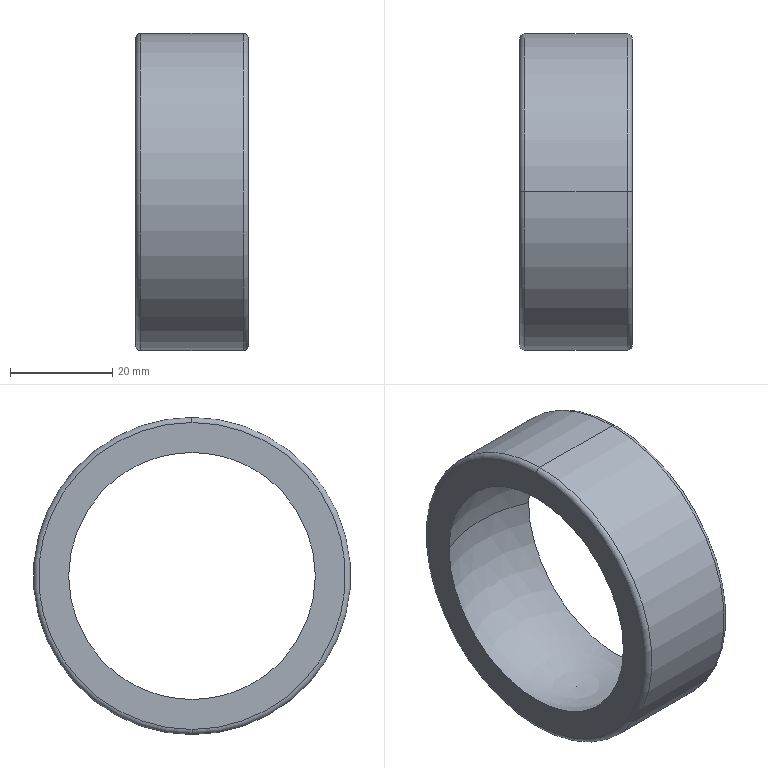Part | SolidWorks | features Fillet 1, Revolution 1 | 1 solid | 10 faces | box 22 x 62 x 62 mm | volume 20588 mm3 | torus 4 | sphere 2 | cylinder 2 | plane 2 | commonest cylinder face diameters 62 x2
STEP:
#1=CARTESIAN_POINT('',(11.,0.,-30.));
#2=VERTEX_POINT('',#1);
#3=CARTESIAN_POINT('',(11.,0.,30.));
#4=VERTEX_POINT('',#3);
#5=CARTESIAN_POINT('',(11.,0.,0.));
#6=DIRECTION('',(1.,0.,0.));
#7=DIRECTION('',(0.,0.,1.));
#8=AXIS2_PLACEMENT_3D('',#5,#6,#7);
#9=CIRCLE('',#8,30.);
#10=EDGE_CURVE('',#2,#4,#9,.T.);
#11=ORIENTED_EDGE('',*,*,#10,.F.);
#12=CARTESIAN_POINT('',(10.,0.,-31.));
#13=VERTEX_POINT('',#12);
#14=CARTESIAN_POINT('',(10.,0.,-30.));
#15=DIRECTION('',(0.,1.,0.));
#16=DIRECTION('',(0.,0.,1.));
#17=AXIS2_PLACEMENT_3D('',#14,#15,#16);
#18=CIRCLE('',#17,1.);
#19=EDGE_CURVE('',#2,#13,#18,.T.);
#20=ORIENTED_EDGE('',*,*,#19,.T.);
#21=CARTESIAN_POINT('',(10.,0.,31.));
#22=VERTEX_POINT('',#21);
#23=CARTESIAN_POINT('',(10.,0.,0.));
#24=DIRECTION('',(-1.,0.,0.));
#25=DIRECTION('',(0.,0.,1.));
#26=AXIS2_PLACEMENT_3D('',#23,#24,#25);
#27=CIRCLE('',#26,31.);
#28=EDGE_CURVE('',#22,#13,#27,.T.);
#29=ORIENTED_EDGE('',*,*,#28,.F.);
#30=CARTESIAN_POINT('',(10.,0.,30.));
#31=DIRECTION('',(0.,-1.,0.));
#32=DIRECTION('',(0.,0.,-1.));
#33=AXIS2_PLACEMENT_3D('',#30,#31,#32);
#34=CIRCLE('',#33,1.);
#35=EDGE_CURVE('',#4,#22,#34,.T.);
#36=ORIENTED_EDGE('',*,*,#35,.F.);
#37=EDGE_LOOP('',(#11,#20,#29,#36));
#38=FACE_OUTER_BOUND('',#37,.T.);
#39=CARTESIAN_POINT('',(10.,0.,0.));
#40=DIRECTION('',(-1.,0.,0.));
#41=DIRECTION('',(0.,0.,1.));
#42=AXIS2_PLACEMENT_3D('',#39,#40,#41);
#43=TOROIDAL_SURFACE('',#42,30.,1.);
#44=ADVANCED_FACE('',(#38),#43,.T.);
#45=CARTESIAN_POINT('',(-11.,0.,30.));
#46=VERTEX_POINT('',#45);
#47=CARTESIAN_POINT('',(-11.,0.,-30.));
#48=VERTEX_POINT('',#47);
#49=CARTESIAN_POINT('',(-11.,0.,0.));
#50=DIRECTION('',(-1.,0.,0.));
#51=DIRECTION('',(0.,0.,-1.));
#52=AXIS2_PLACEMENT_3D('',#49,#50,#51);
#53=CIRCLE('',#52,30.);
#54=EDGE_CURVE('',#46,#48,#53,.T.);
#55=ORIENTED_EDGE('',*,*,#54,.F.);
#56=CARTESIAN_POINT('',(-10.,0.,31.));
#57=VERTEX_POINT('',#56);
#58=CARTESIAN_POINT('',(-10.,0.,30.));
#59=DIRECTION('',(0.,1.,0.));
#60=DIRECTION('',(0.,0.,1.));
#61=AXIS2_PLACEMENT_3D('',#58,#59,#60);
#62=CIRCLE('',#61,1.);
#63=EDGE_CURVE('',#46,#57,#62,.T.);
#64=ORIENTED_EDGE('',*,*,#63,.T.);
#65=CARTESIAN_POINT('',(-10.,0.,-31.));
#66=VERTEX_POINT('',#65);
#67=CARTESIAN_POINT('',(-10.,0.,0.));
#68=DIRECTION('',(1.,0.,0.));
#69=DIRECTION('',(0.,0.,-1.));
#70=AXIS2_PLACEMENT_3D('',#67,#68,#69);
#71=CIRCLE('',#70,31.);
#72=EDGE_CURVE('',#66,#57,#71,.T.);
#73=ORIENTED_EDGE('',*,*,#72,.F.);
#74=CARTESIAN_POINT('',(-10.,0.,-30.));
#75=DIRECTION('',(0.,-1.,0.));
#76=DIRECTION('',(0.,0.,-1.));
#77=AXIS2_PLACEMENT_3D('',#74,#75,#76);
#78=CIRCLE('',#77,1.);
#79=EDGE_CURVE('',#48,#66,#78,.T.);
#80=ORIENTED_EDGE('',*,*,#79,.F.);
#81=EDGE_LOOP('',(#55,#64,#73,#80));
#82=FACE_OUTER_BOUND('',#81,.T.);
#83=CARTESIAN_POINT('',(-10.,0.,0.));
#84=DIRECTION('',(1.,0.,0.));
#85=DIRECTION('',(0.,0.,-1.));
#86=AXIS2_PLACEMENT_3D('',#83,#84,#85);
#87=TOROIDAL_SURFACE('',#86,30.,1.);
#88=ADVANCED_FACE('',(#82),#87,.T.);
#89=CARTESIAN_POINT('',(11.,-24.109,0.));
#90=VERTEX_POINT('',#89);
#91=CARTESIAN_POINT('',(11.,24.109,0.));
#92=VERTEX_POINT('',#91);
#93=CARTESIAN_POINT('',(11.,0.,0.));
#94=DIRECTION('',(-1.,0.,0.));
#95=DIRECTION('',(0.,0.,1.));
#96=AXIS2_PLACEMENT_3D('',#93,#94,#95);
#97=CIRCLE('',#96,24.109);
#98=EDGE_CURVE('',#90,#92,#97,.T.);
#99=ORIENTED_EDGE('',*,*,#98,.F.);
#100=CARTESIAN_POINT('',(-11.,-24.109,0.));
#101=VERTEX_POINT('',#100);
#102=CARTESIAN_POINT('',(0.,0.,0.));
#103=DIRECTION('',(0.,0.,-1.));
#104=DIRECTION('',(0.,1.,0.));
#105=AXIS2_PLACEMENT_3D('',#102,#103,#104);
#106=CIRCLE('',#105,26.5);
#107=EDGE_CURVE('',#90,#101,#106,.T.);
#108=ORIENTED_EDGE('',*,*,#107,.T.);
#109=CARTESIAN_POINT('',(-11.,24.109,0.));
#110=VERTEX_POINT('',#109);
#111=CARTESIAN_POINT('',(-11.,0.,0.));
#112=DIRECTION('',(-1.,0.,0.));
#113=DIRECTION('',(0.,0.,1.));
#114=AXIS2_PLACEMENT_3D('',#111,#112,#113);
#115=CIRCLE('',#114,24.109);
#116=EDGE_CURVE('',#101,#110,#115,.T.);
#117=ORIENTED_EDGE('',*,*,#116,.T.);
#118=CARTESIAN_POINT('',(0.,0.,0.));
#119=DIRECTION('',(0.,0.,1.));
#120=DIRECTION('',(1.,0.,0.));
#121=AXIS2_PLACEMENT_3D('',#118,#119,#120);
#122=CIRCLE('',#121,26.5);
#123=EDGE_CURVE('',#92,#110,#122,.T.);
#124=ORIENTED_EDGE('',*,*,#123,.F.);
#125=EDGE_LOOP('',(#99,#108,#117,#124));
#126=FACE_OUTER_BOUND('',#125,.T.);
#127=CARTESIAN_POINT('',(0.,0.,0.));
#128=DIRECTION('',(0.,0.,-1.));
#129=DIRECTION('',(0.,1.,0.));
#130=AXIS2_PLACEMENT_3D('',#127,#128,#129);
#131=SPHERICAL_SURFACE('',#130,26.5);
#132=ADVANCED_FACE('',(#126),#131,.F.);
#133=ORIENTED_EDGE('',*,*,#28,.T.);
#134=CARTESIAN_POINT('',(-53.013,0.,-31.));
#135=DIRECTION('',(-1.,0.,0.));
#136=VECTOR('',#135,1000.);
#137=LINE('',#134,#136);
#138=EDGE_CURVE('',#13,#66,#137,.T.);
#139=ORIENTED_EDGE('',*,*,#138,.T.);
#140=ORIENTED_EDGE('',*,*,#72,.T.);
#141=CARTESIAN_POINT('',(-53.013,0.,31.));
#142=DIRECTION('',(-1.,0.,0.));
#143=VECTOR('',#142,1000.);
#144=LINE('',#141,#143);
#145=EDGE_CURVE('',#22,#57,#144,.T.);
#146=ORIENTED_EDGE('',*,*,#145,.F.);
#147=EDGE_LOOP('',(#133,#139,#140,#146));
#148=FACE_OUTER_BOUND('',#147,.T.);
#149=CARTESIAN_POINT('',(-53.013,0.,0.));
#150=DIRECTION('',(-1.,0.,0.));
#151=DIRECTION('',(0.,0.,1.));
#152=AXIS2_PLACEMENT_3D('',#149,#150,#151);
#153=CYLINDRICAL_SURFACE('',#152,31.);
#154=ADVANCED_FACE('',(#148),#153,.T.);
#155=ORIENTED_EDGE('',*,*,#138,.F.);
#156=CARTESIAN_POINT('',(10.,0.,0.));
#157=DIRECTION('',(-1.,0.,0.));
#158=DIRECTION('',(0.,0.,1.));
#159=AXIS2_PLACEMENT_3D('',#156,#157,#158);
#160=CIRCLE('',#159,31.);
#161=EDGE_CURVE('',#13,#22,#160,.T.);
#162=ORIENTED_EDGE('',*,*,#161,.T.);
#163=ORIENTED_EDGE('',*,*,#145,.T.);
#164=CARTESIAN_POINT('',(-10.,0.,0.));
#165=DIRECTION('',(1.,0.,0.));
#166=DIRECTION('',(0.,0.,-1.));
#167=AXIS2_PLACEMENT_3D('',#164,#165,#166);
#168=CIRCLE('',#167,31.);
#169=EDGE_CURVE('',#57,#66,#168,.T.);
#170=ORIENTED_EDGE('',*,*,#169,.T.);
#171=EDGE_LOOP('',(#155,#162,#163,#170));
#172=FACE_OUTER_BOUND('',#171,.T.);
#173=CARTESIAN_POINT('',(-53.013,0.,0.));
#174=DIRECTION('',(-1.,0.,0.));
#175=DIRECTION('',(0.,0.,1.));
#176=AXIS2_PLACEMENT_3D('',#173,#174,#175);
#177=CYLINDRICAL_SURFACE('',#176,31.);
#178=ADVANCED_FACE('',(#172),#177,.T.);
#179=CARTESIAN_POINT('',(-11.,0.,0.));
#180=DIRECTION('',(-1.,0.,0.));
#181=DIRECTION('',(0.,0.,-1.));
#182=AXIS2_PLACEMENT_3D('',#179,#180,#181);
#183=CIRCLE('',#182,30.);
#184=EDGE_CURVE('',#48,#46,#183,.T.);
#185=ORIENTED_EDGE('',*,*,#184,.T.);
#186=ORIENTED_EDGE('',*,*,#54,.T.);
#187=EDGE_LOOP('',(#185,#186));
#188=FACE_OUTER_BOUND('',#187,.T.);
#189=CARTESIAN_POINT('',(-11.,0.,0.));
#190=DIRECTION('',(-1.,0.,0.));
#191=DIRECTION('',(0.,0.,1.));
#192=AXIS2_PLACEMENT_3D('',#189,#190,#191);
#193=CIRCLE('',#192,24.109);
#194=EDGE_CURVE('',#110,#101,#193,.T.);
#195=ORIENTED_EDGE('',*,*,#194,.F.);
#196=ORIENTED_EDGE('',*,*,#116,.F.);
#197=EDGE_LOOP('',(#195,#196));
#198=FACE_BOUND('',#197,.T.);
#199=CARTESIAN_POINT('',(-11.,31.,0.));
#200=DIRECTION('',(1.,0.,0.));
#201=DIRECTION('',(0.,0.,-1.));
#202=AXIS2_PLACEMENT_3D('',#199,#200,#201);
#203=PLANE('',#202);
#204=ADVANCED_FACE('',(#188,#198),#203,.F.);
#205=ORIENTED_EDGE('',*,*,#107,.F.);
#206=CARTESIAN_POINT('',(11.,0.,0.));
#207=DIRECTION('',(-1.,0.,0.));
#208=DIRECTION('',(0.,0.,1.));
#209=AXIS2_PLACEMENT_3D('',#206,#207,#208);
#210=CIRCLE('',#209,24.109);
#211=EDGE_CURVE('',#92,#90,#210,.T.);
#212=ORIENTED_EDGE('',*,*,#211,.F.);
#213=ORIENTED_EDGE('',*,*,#123,.T.);
#214=ORIENTED_EDGE('',*,*,#194,.T.);
#215=EDGE_LOOP('',(#205,#212,#213,#214));
#216=FACE_OUTER_BOUND('',#215,.T.);
#217=CARTESIAN_POINT('',(0.,0.,0.));
#218=DIRECTION('',(0.,0.,-1.));
#219=DIRECTION('',(0.,1.,0.));
#220=AXIS2_PLACEMENT_3D('',#217,#218,#219);
#221=SPHERICAL_SURFACE('',#220,26.5);
#222=ADVANCED_FACE('',(#216),#221,.F.);
#223=CARTESIAN_POINT('',(11.,0.,0.));
#224=DIRECTION('',(1.,0.,0.));
#225=DIRECTION('',(0.,0.,1.));
#226=AXIS2_PLACEMENT_3D('',#223,#224,#225);
#227=CIRCLE('',#226,30.);
#228=EDGE_CURVE('',#4,#2,#227,.T.);
#229=ORIENTED_EDGE('',*,*,#228,.T.);
#230=ORIENTED_EDGE('',*,*,#10,.T.);
#231=EDGE_LOOP('',(#229,#230));
#232=FACE_OUTER_BOUND('',#231,.T.);
#233=ORIENTED_EDGE('',*,*,#211,.T.);
#234=ORIENTED_EDGE('',*,*,#98,.T.);
#235=EDGE_LOOP('',(#233,#234));
#236=FACE_BOUND('',#235,.T.);
#237=CARTESIAN_POINT('',(11.,31.,0.));
#238=DIRECTION('',(-1.,0.,0.));
#239=DIRECTION('',(0.,0.,1.));
#240=AXIS2_PLACEMENT_3D('',#237,#238,#239);
#241=PLANE('',#240);
#242=ADVANCED_FACE('',(#232,#236),#241,.F.);
#243=ORIENTED_EDGE('',*,*,#63,.F.);
#244=ORIENTED_EDGE('',*,*,#184,.F.);
#245=ORIENTED_EDGE('',*,*,#79,.T.);
#246=ORIENTED_EDGE('',*,*,#169,.F.);
#247=EDGE_LOOP('',(#243,#244,#245,#246));
#248=FACE_OUTER_BOUND('',#247,.T.);
#249=CARTESIAN_POINT('',(-10.,0.,0.));
#250=DIRECTION('',(1.,0.,0.));
#251=DIRECTION('',(0.,0.,-1.));
#252=AXIS2_PLACEMENT_3D('',#249,#250,#251);
#253=TOROIDAL_SURFACE('',#252,30.,1.);
#254=ADVANCED_FACE('',(#248),#253,.T.);
#255=ORIENTED_EDGE('',*,*,#19,.F.);
#256=ORIENTED_EDGE('',*,*,#228,.F.);
#257=ORIENTED_EDGE('',*,*,#35,.T.);
#258=ORIENTED_EDGE('',*,*,#161,.F.);
#259=EDGE_LOOP('',(#255,#256,#257,#258));
#260=FACE_OUTER_BOUND('',#259,.T.);
#261=CARTESIAN_POINT('',(10.,0.,0.));
#262=DIRECTION('',(-1.,0.,0.));
#263=DIRECTION('',(0.,0.,1.));
#264=AXIS2_PLACEMENT_3D('',#261,#262,#263);
#265=TOROIDAL_SURFACE('',#264,30.,1.);
#266=ADVANCED_FACE('',(#260),#265,.T.);
#267=CLOSED_SHELL('',(#44,#88,#132,#154,#178,#204,#222,#242,#254,#266));
#268=MANIFOLD_SOLID_BREP('',#267);
#269=CARTESIAN_POINT('',(0.,0.,0.));
#270=DIRECTION('',(0.,0.,1.));
#271=DIRECTION('',(1.,0.,0.));
#272=AXIS2_PLACEMENT_3D('',#269,#270,#271);
#273=(LENGTH_UNIT()NAMED_UNIT(*)SI_UNIT(.MILLI.,.METRE.));
#274=UNCERTAINTY_MEASURE_WITH_UNIT(LENGTH_MEASURE(0.00001),#273,'','');
#275=(NAMED_UNIT(*)PLANE_ANGLE_UNIT()SI_UNIT($,.RADIAN.));
#276=(NAMED_UNIT(*)SI_UNIT($,.STERADIAN.)SOLID_ANGLE_UNIT());
#277=(GEOMETRIC_REPRESENTATION_CONTEXT(3)GLOBAL_UNCERTAINTY_ASSIGNED_CONTEXT((#274))GLOBAL_UNIT_ASSIGNED_CONTEXT((#273,#275,#276))REPRESENTATION_CONTEXT('',''));
#278=ADVANCED_BREP_SHAPE_REPRESENTATION('',(#268,#272),#277);